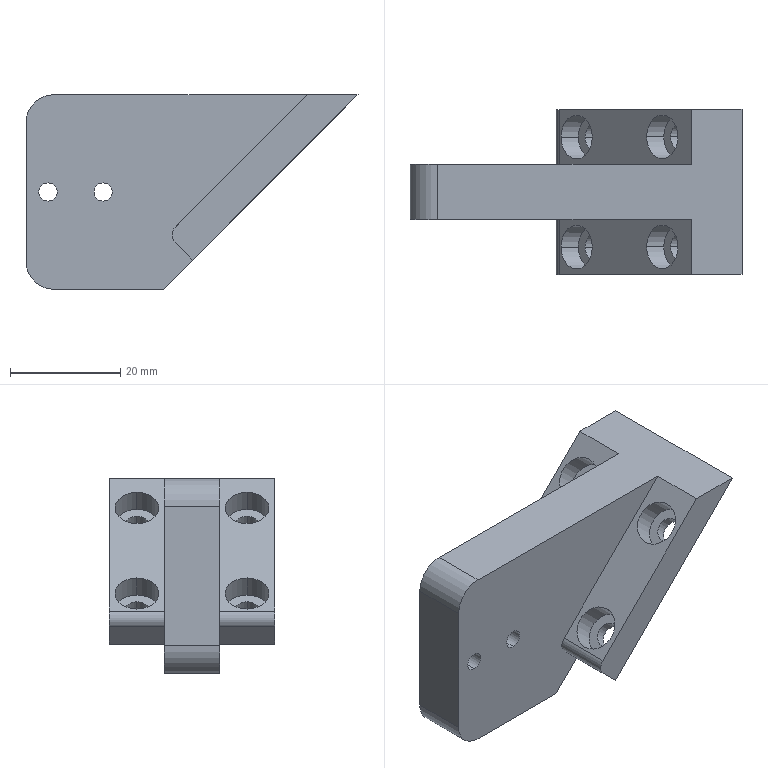Part | SolidWorks | features Fillet 2, HoleWzd 2, Extrusion 1, ICE 1, MirrorPattern 1 | 1 solid | 40 faces | box 60.355 x 30 x 35.355 mm | volume 18878 mm3 | cylinder 24 | plane 16 | commonest cylinder face diameters 4.5 x8 8 x8 3.3 x4 4 x2 10 x2
STEP:
#1=CARTESIAN_POINT('',(18.586,10.,-11.799));
#2=VERTEX_POINT('',#1);
#3=CARTESIAN_POINT('',(24.243,10.,-6.142));
#4=VERTEX_POINT('',#3);
#5=CARTESIAN_POINT('',(21.415,10.,-8.971));
#6=DIRECTION('',(-0.7071,0.,0.7071));
#7=DIRECTION('',(0.7071,0.,0.7071));
#8=AXIS2_PLACEMENT_3D('',#5,#6,#7);
#9=CIRCLE('',#8,4.);
#10=EDGE_CURVE('',#2,#4,#9,.T.);
#11=ORIENTED_EDGE('',*,*,#10,.F.);
#12=CARTESIAN_POINT('',(15.475,10.,-8.688));
#13=VERTEX_POINT('',#12);
#14=CARTESIAN_POINT('',(15.475,10.,-8.688));
#15=DIRECTION('',(-0.7071,0.,0.7071));
#16=VECTOR('',#15,1000.);
#17=LINE('',#14,#16);
#18=EDGE_CURVE('',#2,#13,#17,.T.);
#19=ORIENTED_EDGE('',*,*,#18,.T.);
#20=CARTESIAN_POINT('',(21.132,10.,-3.031));
#21=VERTEX_POINT('',#20);
#22=CARTESIAN_POINT('',(18.303,10.,-5.86));
#23=DIRECTION('',(-0.7071,0.,0.7071));
#24=DIRECTION('',(0.7071,0.,0.7071));
#25=AXIS2_PLACEMENT_3D('',#22,#23,#24);
#26=CIRCLE('',#25,4.);
#27=EDGE_CURVE('',#13,#21,#26,.T.);
#28=ORIENTED_EDGE('',*,*,#27,.T.);
#29=CARTESIAN_POINT('',(21.132,10.,-3.031));
#30=DIRECTION('',(-0.7071,0.,0.7071));
#31=VECTOR('',#30,1000.);
#32=LINE('',#29,#31);
#33=EDGE_CURVE('',#4,#21,#32,.T.);
#34=ORIENTED_EDGE('',*,*,#33,.F.);
#35=EDGE_LOOP('',(#11,#19,#28,#34));
#36=FACE_OUTER_BOUND('',#35,.T.);
#37=CARTESIAN_POINT('',(18.303,10.,-5.86));
#38=DIRECTION('',(-0.7071,0.,0.7071));
#39=DIRECTION('',(0.7071,0.,0.7071));
#40=AXIS2_PLACEMENT_3D('',#37,#38,#39);
#41=CYLINDRICAL_SURFACE('',#40,4.);
#42=ADVANCED_FACE('',(#36),#41,.F.);
#43=CARTESIAN_POINT('',(21.309,10.,-12.047));
#44=VERTEX_POINT('',#43);
#45=CARTESIAN_POINT('',(24.49,10.,-8.865));
#46=VERTEX_POINT('',#45);
#47=CARTESIAN_POINT('',(22.899,10.,-10.456));
#48=DIRECTION('',(-0.7071,0.,0.7071));
#49=DIRECTION('',(0.7071,0.,0.7071));
#50=AXIS2_PLACEMENT_3D('',#47,#48,#49);
#51=CIRCLE('',#50,2.25);
#52=EDGE_CURVE('',#44,#46,#51,.T.);
#53=ORIENTED_EDGE('',*,*,#52,.F.);
#54=CARTESIAN_POINT('',(19.824,10.,-10.562));
#55=VERTEX_POINT('',#54);
#56=CARTESIAN_POINT('',(16.712,10.,-7.451));
#57=DIRECTION('',(-0.7071,0.,0.7071));
#58=VECTOR('',#57,1000.);
#59=LINE('',#56,#58);
#60=EDGE_CURVE('',#44,#55,#59,.T.);
#61=ORIENTED_EDGE('',*,*,#60,.T.);
#62=CARTESIAN_POINT('',(23.006,10.,-7.38));
#63=VERTEX_POINT('',#62);
#64=CARTESIAN_POINT('',(21.415,10.,-8.971));
#65=DIRECTION('',(-0.7071,0.,0.7071));
#66=DIRECTION('',(0.7071,0.,0.7071));
#67=AXIS2_PLACEMENT_3D('',#64,#65,#66);
#68=CIRCLE('',#67,2.25);
#69=EDGE_CURVE('',#55,#63,#68,.T.);
#70=ORIENTED_EDGE('',*,*,#69,.T.);
#71=CARTESIAN_POINT('',(19.894,10.,-4.269));
#72=DIRECTION('',(-0.7071,0.,0.7071));
#73=VECTOR('',#72,1000.);
#74=LINE('',#71,#73);
#75=EDGE_CURVE('',#46,#63,#74,.T.);
#76=ORIENTED_EDGE('',*,*,#75,.F.);
#77=EDGE_LOOP('',(#53,#61,#70,#76));
#78=FACE_OUTER_BOUND('',#77,.T.);
#79=CARTESIAN_POINT('',(18.303,10.,-5.86));
#80=DIRECTION('',(-0.7071,0.,0.7071));
#81=DIRECTION('',(0.7071,0.,0.7071));
#82=AXIS2_PLACEMENT_3D('',#79,#80,#81);
#83=CYLINDRICAL_SURFACE('',#82,2.25);
#84=ADVANCED_FACE('',(#78),#83,.F.);
#85=CARTESIAN_POINT('',(34.142,10.,3.757));
#86=VERTEX_POINT('',#85);
#87=CARTESIAN_POINT('',(39.799,10.,9.414));
#88=VERTEX_POINT('',#87);
#89=CARTESIAN_POINT('',(36.971,10.,6.585));
#90=DIRECTION('',(-0.7071,0.,0.7071));
#91=DIRECTION('',(0.7071,0.,0.7071));
#92=AXIS2_PLACEMENT_3D('',#89,#90,#91);
#93=CIRCLE('',#92,4.);
#94=EDGE_CURVE('',#86,#88,#93,.T.);
#95=ORIENTED_EDGE('',*,*,#94,.F.);
#96=CARTESIAN_POINT('',(31.031,10.,6.868));
#97=VERTEX_POINT('',#96);
#98=CARTESIAN_POINT('',(31.031,10.,6.868));
#99=DIRECTION('',(-0.7071,0.,0.7071));
#100=VECTOR('',#99,1000.);
#101=LINE('',#98,#100);
#102=EDGE_CURVE('',#86,#97,#101,.T.);
#103=ORIENTED_EDGE('',*,*,#102,.T.);
#104=CARTESIAN_POINT('',(36.688,10.,12.525));
#105=VERTEX_POINT('',#104);
#106=CARTESIAN_POINT('',(33.86,10.,9.697));
#107=DIRECTION('',(-0.7071,0.,0.7071));
#108=DIRECTION('',(0.7071,0.,0.7071));
#109=AXIS2_PLACEMENT_3D('',#106,#107,#108);
#110=CIRCLE('',#109,4.);
#111=EDGE_CURVE('',#97,#105,#110,.T.);
#112=ORIENTED_EDGE('',*,*,#111,.T.);
#113=CARTESIAN_POINT('',(36.688,10.,12.525));
#114=DIRECTION('',(-0.7071,0.,0.7071));
#115=VECTOR('',#114,1000.);
#116=LINE('',#113,#115);
#117=EDGE_CURVE('',#88,#105,#116,.T.);
#118=ORIENTED_EDGE('',*,*,#117,.F.);
#119=EDGE_LOOP('',(#95,#103,#112,#118));
#120=FACE_OUTER_BOUND('',#119,.T.);
#121=CARTESIAN_POINT('',(33.86,10.,9.697));
#122=DIRECTION('',(-0.7071,0.,0.7071));
#123=DIRECTION('',(0.7071,0.,0.7071));
#124=AXIS2_PLACEMENT_3D('',#121,#122,#123);
#125=CYLINDRICAL_SURFACE('',#124,4.);
#126=ADVANCED_FACE('',(#120),#125,.F.);
#127=CARTESIAN_POINT('',(36.865,10.,3.51));
#128=VERTEX_POINT('',#127);
#129=CARTESIAN_POINT('',(40.047,10.,6.691));
#130=VERTEX_POINT('',#129);
#131=CARTESIAN_POINT('',(38.456,10.,5.101));
#132=DIRECTION('',(-0.7071,0.,0.7071));
#133=DIRECTION('',(0.7071,0.,0.7071));
#134=AXIS2_PLACEMENT_3D('',#131,#132,#133);
#135=CIRCLE('',#134,2.25);
#136=EDGE_CURVE('',#128,#130,#135,.T.);
#137=ORIENTED_EDGE('',*,*,#136,.F.);
#138=CARTESIAN_POINT('',(35.38,10.,4.994));
#139=VERTEX_POINT('',#138);
#140=CARTESIAN_POINT('',(32.269,10.,8.106));
#141=DIRECTION('',(-0.7071,0.,0.7071));
#142=VECTOR('',#141,1000.);
#143=LINE('',#140,#142);
#144=EDGE_CURVE('',#128,#139,#143,.T.);
#145=ORIENTED_EDGE('',*,*,#144,.T.);
#146=CARTESIAN_POINT('',(38.562,10.,8.176));
#147=VERTEX_POINT('',#146);
#148=CARTESIAN_POINT('',(36.971,10.,6.585));
#149=DIRECTION('',(-0.7071,0.,0.7071));
#150=DIRECTION('',(0.7071,0.,0.7071));
#151=AXIS2_PLACEMENT_3D('',#148,#149,#150);
#152=CIRCLE('',#151,2.25);
#153=EDGE_CURVE('',#139,#147,#152,.T.);
#154=ORIENTED_EDGE('',*,*,#153,.T.);
#155=CARTESIAN_POINT('',(35.451,10.,11.288));
#156=DIRECTION('',(-0.7071,0.,0.7071));
#157=VECTOR('',#156,1000.);
#158=LINE('',#155,#157);
#159=EDGE_CURVE('',#130,#147,#158,.T.);
#160=ORIENTED_EDGE('',*,*,#159,.F.);
#161=EDGE_LOOP('',(#137,#145,#154,#160));
#162=FACE_OUTER_BOUND('',#161,.T.);
#163=CARTESIAN_POINT('',(33.86,10.,9.697));
#164=DIRECTION('',(-0.7071,0.,0.7071));
#165=DIRECTION('',(0.7071,0.,0.7071));
#166=AXIS2_PLACEMENT_3D('',#163,#164,#165);
#167=CYLINDRICAL_SURFACE('',#166,2.25);
#168=ADVANCED_FACE('',(#162),#167,.F.);
#169=CARTESIAN_POINT('',(18.586,-10.,-11.799));
#170=VERTEX_POINT('',#169);
#171=CARTESIAN_POINT('',(24.243,-10.,-6.142));
#172=VERTEX_POINT('',#171);
#173=CARTESIAN_POINT('',(21.415,-10.,-8.971));
#174=DIRECTION('',(-0.7071,0.,0.7071));
#175=DIRECTION('',(0.7071,0.,0.7071));
#176=AXIS2_PLACEMENT_3D('',#173,#174,#175);
#177=CIRCLE('',#176,4.);
#178=EDGE_CURVE('',#170,#172,#177,.T.);
#179=ORIENTED_EDGE('',*,*,#178,.F.);
#180=CARTESIAN_POINT('',(15.475,-10.,-8.688));
#181=VERTEX_POINT('',#180);
#182=CARTESIAN_POINT('',(15.475,-10.,-8.688));
#183=DIRECTION('',(-0.7071,0.,0.7071));
#184=VECTOR('',#183,1000.);
#185=LINE('',#182,#184);
#186=EDGE_CURVE('',#170,#181,#185,.T.);
#187=ORIENTED_EDGE('',*,*,#186,.T.);
#188=CARTESIAN_POINT('',(21.132,-10.,-3.031));
#189=VERTEX_POINT('',#188);
#190=CARTESIAN_POINT('',(18.303,-10.,-5.86));
#191=DIRECTION('',(-0.7071,0.,0.7071));
#192=DIRECTION('',(0.7071,0.,0.7071));
#193=AXIS2_PLACEMENT_3D('',#190,#191,#192);
#194=CIRCLE('',#193,4.);
#195=EDGE_CURVE('',#181,#189,#194,.T.);
#196=ORIENTED_EDGE('',*,*,#195,.T.);
#197=CARTESIAN_POINT('',(21.132,-10.,-3.031));
#198=DIRECTION('',(-0.7071,0.,0.7071));
#199=VECTOR('',#198,1000.);
#200=LINE('',#197,#199);
#201=EDGE_CURVE('',#172,#189,#200,.T.);
#202=ORIENTED_EDGE('',*,*,#201,.F.);
#203=EDGE_LOOP('',(#179,#187,#196,#202));
#204=FACE_OUTER_BOUND('',#203,.T.);
#205=CARTESIAN_POINT('',(18.303,-10.,-5.86));
#206=DIRECTION('',(-0.7071,0.,0.7071));
#207=DIRECTION('',(0.7071,0.,0.7071));
#208=AXIS2_PLACEMENT_3D('',#205,#206,#207);
#209=CYLINDRICAL_SURFACE('',#208,4.);
#210=ADVANCED_FACE('',(#204),#209,.F.);
#211=CARTESIAN_POINT('',(21.309,-10.,-12.047));
#212=VERTEX_POINT('',#211);
#213=CARTESIAN_POINT('',(24.49,-10.,-8.865));
#214=VERTEX_POINT('',#213);
#215=CARTESIAN_POINT('',(22.899,-10.,-10.456));
#216=DIRECTION('',(-0.7071,0.,0.7071));
#217=DIRECTION('',(0.7071,0.,0.7071));
#218=AXIS2_PLACEMENT_3D('',#215,#216,#217);
#219=CIRCLE('',#218,2.25);
#220=EDGE_CURVE('',#212,#214,#219,.T.);
#221=ORIENTED_EDGE('',*,*,#220,.F.);
#222=CARTESIAN_POINT('',(19.824,-10.,-10.562));
#223=VERTEX_POINT('',#222);
#224=CARTESIAN_POINT('',(16.712,-10.,-7.451));
#225=DIRECTION('',(-0.7071,0.,0.7071));
#226=VECTOR('',#225,1000.);
#227=LINE('',#224,#226);
#228=EDGE_CURVE('',#212,#223,#227,.T.);
#229=ORIENTED_EDGE('',*,*,#228,.T.);
#230=CARTESIAN_POINT('',(23.006,-10.,-7.38));
#231=VERTEX_POINT('',#230);
#232=CARTESIAN_POINT('',(21.415,-10.,-8.971));
#233=DIRECTION('',(-0.7071,0.,0.7071));
#234=DIRECTION('',(0.7071,0.,0.7071));
#235=AXIS2_PLACEMENT_3D('',#232,#233,#234);
#236=CIRCLE('',#235,2.25);
#237=EDGE_CURVE('',#223,#231,#236,.T.);
#238=ORIENTED_EDGE('',*,*,#237,.T.);
#239=CARTESIAN_POINT('',(19.894,-10.,-4.269));
#240=DIRECTION('',(-0.7071,0.,0.7071));
#241=VECTOR('',#240,1000.);
#242=LINE('',#239,#241);
#243=EDGE_CURVE('',#214,#231,#242,.T.);
#244=ORIENTED_EDGE('',*,*,#243,.F.);
#245=EDGE_LOOP('',(#221,#229,#238,#244));
#246=FACE_OUTER_BOUND('',#245,.T.);
#247=CARTESIAN_POINT('',(18.303,-10.,-5.86));
#248=DIRECTION('',(-0.7071,0.,0.7071));
#249=DIRECTION('',(0.7071,0.,0.7071));
#250=AXIS2_PLACEMENT_3D('',#247,#248,#249);
#251=CYLINDRICAL_SURFACE('',#250,2.25);
#252=ADVANCED_FACE('',(#246),#251,.F.);
#253=CARTESIAN_POINT('',(34.142,-10.,3.757));
#254=VERTEX_POINT('',#253);
#255=CARTESIAN_POINT('',(39.799,-10.,9.414));
#256=VERTEX_POINT('',#255);
#257=CARTESIAN_POINT('',(36.971,-10.,6.585));
#258=DIRECTION('',(-0.7071,0.,0.7071));
#259=DIRECTION('',(0.7071,0.,0.7071));
#260=AXIS2_PLACEMENT_3D('',#257,#258,#259);
#261=CIRCLE('',#260,4.);
#262=EDGE_CURVE('',#254,#256,#261,.T.);
#263=ORIENTED_EDGE('',*,*,#262,.F.);
#264=CARTESIAN_POINT('',(31.031,-10.,6.868));
#265=VERTEX_POINT('',#264);
#266=CARTESIAN_POINT('',(31.031,-10.,6.868));
#267=DIRECTION('',(-0.7071,0.,0.7071));
#268=VECTOR('',#267,1000.);
#269=LINE('',#266,#268);
#270=EDGE_CURVE('',#254,#265,#269,.T.);
#271=ORIENTED_EDGE('',*,*,#270,.T.);
#272=CARTESIAN_POINT('',(36.688,-10.,12.525));
#273=VERTEX_POINT('',#272);
#274=CARTESIAN_POINT('',(33.86,-10.,9.697));
#275=DIRECTION('',(-0.7071,0.,0.7071));
#276=DIRECTION('',(0.7071,0.,0.7071));
#277=AXIS2_PLACEMENT_3D('',#274,#275,#276);
#278=CIRCLE('',#277,4.);
#279=EDGE_CURVE('',#265,#273,#278,.T.);
#280=ORIENTED_EDGE('',*,*,#279,.T.);
#281=CARTESIAN_POINT('',(36.688,-10.,12.525));
#282=DIRECTION('',(-0.7071,0.,0.7071));
#283=VECTOR('',#282,1000.);
#284=LINE('',#281,#283);
#285=EDGE_CURVE('',#256,#273,#284,.T.);
#286=ORIENTED_EDGE('',*,*,#285,.F.);
#287=EDGE_LOOP('',(#263,#271,#280,#286));
#288=FACE_OUTER_BOUND('',#287,.T.);
#289=CARTESIAN_POINT('',(33.86,-10.,9.697));
#290=DIRECTION('',(-0.7071,0.,0.7071));
#291=DIRECTION('',(0.7071,0.,0.7071));
#292=AXIS2_PLACEMENT_3D('',#289,#290,#291);
#293=CYLINDRICAL_SURFACE('',#292,4.);
#294=ADVANCED_FACE('',(#288),#293,.F.);
#295=CARTESIAN_POINT('',(36.865,-10.,3.51));
#296=VERTEX_POINT('',#295);
#297=CARTESIAN_POINT('',(40.047,-10.,6.691));
#298=VERTEX_POINT('',#297);
#299=CARTESIAN_POINT('',(38.456,-10.,5.101));
#300=DIRECTION('',(-0.7071,0.,0.7071));
#301=DIRECTION('',(0.7071,0.,0.7071));
#302=AXIS2_PLACEMENT_3D('',#299,#300,#301);
#303=CIRCLE('',#302,2.25);
#304=EDGE_CURVE('',#296,#298,#303,.T.);
#305=ORIENTED_EDGE('',*,*,#304,.F.);
#306=CARTESIAN_POINT('',(35.38,-10.,4.994));
#307=VERTEX_POINT('',#306);
#308=CARTESIAN_POINT('',(32.269,-10.,8.106));
#309=DIRECTION('',(-0.7071,0.,0.7071));
#310=VECTOR('',#309,1000.);
#311=LINE('',#308,#310);
#312=EDGE_CURVE('',#296,#307,#311,.T.);
#313=ORIENTED_EDGE('',*,*,#312,.T.);
#314=CARTESIAN_POINT('',(38.562,-10.,8.176));
#315=VERTEX_POINT('',#314);
#316=CARTESIAN_POINT('',(36.971,-10.,6.585));
#317=DIRECTION('',(-0.7071,0.,0.7071));
#318=DIRECTION('',(0.7071,0.,0.7071));
#319=AXIS2_PLACEMENT_3D('',#316,#317,#318);
#320=CIRCLE('',#319,2.25);
#321=EDGE_CURVE('',#307,#315,#320,.T.);
#322=ORIENTED_EDGE('',*,*,#321,.T.);
#323=CARTESIAN_POINT('',(35.451,-10.,11.288));
#324=DIRECTION('',(-0.7071,0.,0.7071));
#325=VECTOR('',#324,1000.);
#326=LINE('',#323,#325);
#327=EDGE_CURVE('',#298,#315,#326,.T.);
#328=ORIENTED_EDGE('',*,*,#327,.F.);
#329=EDGE_LOOP('',(#305,#313,#322,#328));
#330=FACE_OUTER_BOUND('',#329,.T.);
#331=CARTESIAN_POINT('',(33.86,-10.,9.697));
#332=DIRECTION('',(-0.7071,0.,0.7071));
#333=DIRECTION('',(0.7071,0.,0.7071));
#334=AXIS2_PLACEMENT_3D('',#331,#332,#333);
#335=CYLINDRICAL_SURFACE('',#334,2.25);
#336=ADVANCED_FACE('',(#330),#335,.F.);
#337=CARTESIAN_POINT('',(-8.,5.,-1.028));
#338=VERTEX_POINT('',#337);
#339=CARTESIAN_POINT('',(-8.,5.,-4.328));
#340=VERTEX_POINT('',#339);
#341=CARTESIAN_POINT('',(-8.,5.,-2.678));
#342=DIRECTION('',(0.,-1.,0.));
#343=DIRECTION('',(0.,0.,-1.));
#344=AXIS2_PLACEMENT_3D('',#341,#342,#343);
#345=CIRCLE('',#344,1.65);
#346=EDGE_CURVE('',#338,#340,#345,.T.);
#347=ORIENTED_EDGE('',*,*,#346,.F.);
#348=CARTESIAN_POINT('',(-8.,-5.,-1.028));
#349=VERTEX_POINT('',#348);
#350=CARTESIAN_POINT('',(-8.,-5.,-1.028));
#351=DIRECTION('',(0.,-1.,0.));
#352=VECTOR('',#351,1000.);
#353=LINE('',#350,#352);
#354=EDGE_CURVE('',#338,#349,#353,.T.);
#355=ORIENTED_EDGE('',*,*,#354,.T.);
#356=CARTESIAN_POINT('',(-8.,-5.,-4.328));
#357=VERTEX_POINT('',#356);
#358=CARTESIAN_POINT('',(-8.,-5.,-2.678));
#359=DIRECTION('',(0.,-1.,0.));
#360=DIRECTION('',(0.,0.,-1.));
#361=AXIS2_PLACEMENT_3D('',#358,#359,#360);
#362=CIRCLE('',#361,1.65);
#363=EDGE_CURVE('',#349,#357,#362,.T.);
#364=ORIENTED_EDGE('',*,*,#363,.T.);
#365=CARTESIAN_POINT('',(-8.,-5.,-4.328));
#366=DIRECTION('',(0.,-1.,0.));
#367=VECTOR('',#366,1000.);
#368=LINE('',#365,#367);
#369=EDGE_CURVE('',#340,#357,#368,.T.);
#370=ORIENTED_EDGE('',*,*,#369,.F.);
#371=EDGE_LOOP('',(#347,#355,#364,#370));
#372=FACE_OUTER_BOUND('',#371,.T.);
#373=CARTESIAN_POINT('',(-8.,-5.,-2.678));
#374=DIRECTION('',(0.,-1.,0.));
#375=DIRECTION('',(0.,0.,-1.));
#376=AXIS2_PLACEMENT_3D('',#373,#374,#375);
#377=CYLINDRICAL_SURFACE('',#376,1.65);
#378=ADVANCED_FACE('',(#372),#377,.F.);
#379=CARTESIAN_POINT('',(2.,5.,-1.028));
#380=VERTEX_POINT('',#379);
#381=CARTESIAN_POINT('',(2.,5.,-4.328));
#382=VERTEX_POINT('',#381);
#383=CARTESIAN_POINT('',(2.,5.,-2.678));
#384=DIRECTION('',(0.,-1.,0.));
#385=DIRECTION('',(0.,0.,-1.));
#386=AXIS2_PLACEMENT_3D('',#383,#384,#385);
#387=CIRCLE('',#386,1.65);
#388=EDGE_CURVE('',#380,#382,#387,.T.);
#389=ORIENTED_EDGE('',*,*,#388,.F.);
#390=CARTESIAN_POINT('',(2.,-5.,-1.028));
#391=VERTEX_POINT('',#390);
#392=CARTESIAN_POINT('',(2.,-5.,-1.028));
#393=DIRECTION('',(0.,-1.,0.));
#394=VECTOR('',#393,1000.);
#395=LINE('',#392,#394);
#396=EDGE_CURVE('',#380,#391,#395,.T.);
#397=ORIENTED_EDGE('',*,*,#396,.T.);
#398=CARTESIAN_POINT('',(2.,-5.,-4.328));
#399=VERTEX_POINT('',#398);
#400=CARTESIAN_POINT('',(2.,-5.,-2.678));
#401=DIRECTION('',(0.,-1.,0.));
#402=DIRECTION('',(0.,0.,-1.));
#403=AXIS2_PLACEMENT_3D('',#400,#401,#402);
#404=CIRCLE('',#403,1.65);
#405=EDGE_CURVE('',#391,#399,#404,.T.);
#406=ORIENTED_EDGE('',*,*,#405,.T.);
#407=CARTESIAN_POINT('',(2.,-5.,-4.328));
#408=DIRECTION('',(0.,-1.,0.));
#409=VECTOR('',#408,1000.);
#410=LINE('',#407,#409);
#411=EDGE_CURVE('',#382,#399,#410,.T.);
#412=ORIENTED_EDGE('',*,*,#411,.F.);
#413=EDGE_LOOP('',(#389,#397,#406,#412));
#414=FACE_OUTER_BOUND('',#413,.T.);
#415=CARTESIAN_POINT('',(2.,-5.,-2.678));
#416=DIRECTION('',(0.,-1.,0.));
#417=DIRECTION('',(0.,0.,-1.));
#418=AXIS2_PLACEMENT_3D('',#415,#416,#417);
#419=CYLINDRICAL_SURFACE('',#418,1.65);
#420=ADVANCED_FACE('',(#414),#419,.F.);
#421=CARTESIAN_POINT('',(-8.,5.,-2.678));
#422=DIRECTION('',(0.,-1.,0.));
#423=DIRECTION('',(0.,0.,-1.));
#424=AXIS2_PLACEMENT_3D('',#421,#422,#423);
#425=CIRCLE('',#424,1.65);
#426=EDGE_CURVE('',#340,#338,#425,.T.);
#427=ORIENTED_EDGE('',*,*,#426,.T.);
#428=ORIENTED_EDGE('',*,*,#346,.T.);
#429=EDGE_LOOP('',(#427,#428));
#430=FACE_BOUND('',#429,.T.);
#431=CARTESIAN_POINT('',(2.,5.,-2.678));
#432=DIRECTION('',(0.,-1.,0.));
#433=DIRECTION('',(0.,0.,-1.));
#434=AXIS2_PLACEMENT_3D('',#431,#432,#433);
#435=CIRCLE('',#434,1.65);
#436=EDGE_CURVE('',#382,#380,#435,.T.);
#437=ORIENTED_EDGE('',*,*,#436,.T.);
#438=ORIENTED_EDGE('',*,*,#388,.T.);
#439=EDGE_LOOP('',(#437,#438));
#440=FACE_BOUND('',#439,.T.);
#441=CARTESIAN_POINT('',(-12.,5.,-15.355));
#442=VERTEX_POINT('',#441);
#443=CARTESIAN_POINT('',(-12.,5.,10.));
#444=VERTEX_POINT('',#443);
#445=CARTESIAN_POINT('',(-12.,5.,-20.355));
#446=DIRECTION('',(0.,0.,1.));
#447=VECTOR('',#446,1000.);
#448=LINE('',#445,#447);
#449=EDGE_CURVE('',#442,#444,#448,.T.);
#450=ORIENTED_EDGE('',*,*,#449,.T.);
#451=CARTESIAN_POINT('',(-7.,5.,15.));
#452=VERTEX_POINT('',#451);
#453=CARTESIAN_POINT('',(-7.,5.,10.));
#454=DIRECTION('',(0.,1.,0.));
#455=DIRECTION('',(0.,0.,1.));
#456=AXIS2_PLACEMENT_3D('',#453,#454,#455);
#457=CIRCLE('',#456,5.);
#458=EDGE_CURVE('',#444,#452,#457,.T.);
#459=ORIENTED_EDGE('',*,*,#458,.T.);
#460=CARTESIAN_POINT('',(39.163,5.,15.));
#461=VERTEX_POINT('',#460);
#462=CARTESIAN_POINT('',(-12.,5.,15.));
#463=DIRECTION('',(1.,0.,0.));
#464=VECTOR('',#463,1000.);
#465=LINE('',#462,#464);
#466=EDGE_CURVE('',#452,#461,#465,.T.);
#467=ORIENTED_EDGE('',*,*,#466,.T.);
#468=CARTESIAN_POINT('',(15.121,5.,-9.042));
#469=VERTEX_POINT('',#468);
#470=CARTESIAN_POINT('',(13.707,5.,-10.456));
#471=DIRECTION('',(-0.7071,0.,-0.7071));
#472=VECTOR('',#471,1000.);
#473=LINE('',#470,#472);
#474=EDGE_CURVE('',#461,#469,#473,.T.);
#475=ORIENTED_EDGE('',*,*,#474,.T.);
#476=CARTESIAN_POINT('',(15.121,5.,-11.87));
#477=VERTEX_POINT('',#476);
#478=CARTESIAN_POINT('',(16.536,5.,-10.456));
#479=DIRECTION('',(0.,-1.,0.));
#480=DIRECTION('',(0.,0.,1.));
#481=AXIS2_PLACEMENT_3D('',#478,#479,#480);
#482=CIRCLE('',#481,2.);
#483=EDGE_CURVE('',#469,#477,#482,.T.);
#484=ORIENTED_EDGE('',*,*,#483,.T.);
#485=CARTESIAN_POINT('',(18.303,5.,-15.052));
#486=VERTEX_POINT('',#485);
#487=CARTESIAN_POINT('',(18.303,5.,-15.052));
#488=DIRECTION('',(0.7071,0.,-0.7071));
#489=VECTOR('',#488,1000.);
#490=LINE('',#487,#489);
#491=EDGE_CURVE('',#477,#486,#490,.T.);
#492=ORIENTED_EDGE('',*,*,#491,.T.);
#493=CARTESIAN_POINT('',(13.,5.,-20.355));
#494=VERTEX_POINT('',#493);
#495=CARTESIAN_POINT('',(48.355,5.,15.));
#496=DIRECTION('',(-0.7071,0.,-0.7071));
#497=VECTOR('',#496,1000.);
#498=LINE('',#495,#497);
#499=EDGE_CURVE('',#486,#494,#498,.T.);
#500=ORIENTED_EDGE('',*,*,#499,.T.);
#501=CARTESIAN_POINT('',(-7.,5.,-20.355));
#502=VERTEX_POINT('',#501);
#503=CARTESIAN_POINT('',(13.,5.,-20.355));
#504=DIRECTION('',(-1.,0.,0.));
#505=VECTOR('',#504,1000.);
#506=LINE('',#503,#505);
#507=EDGE_CURVE('',#494,#502,#506,.T.);
#508=ORIENTED_EDGE('',*,*,#507,.T.);
#509=CARTESIAN_POINT('',(-7.,5.,-15.355));
#510=DIRECTION('',(0.,1.,0.));
#511=DIRECTION('',(0.,0.,1.));
#512=AXIS2_PLACEMENT_3D('',#509,#510,#511);
#513=CIRCLE('',#512,5.);
#514=EDGE_CURVE('',#502,#442,#513,.T.);
#515=ORIENTED_EDGE('',*,*,#514,.T.);
#516=EDGE_LOOP('',(#450,#459,#467,#475,#484,#492,#500,#508,#515));
#517=FACE_OUTER_BOUND('',#516,.T.);
#518=CARTESIAN_POINT('',(0.,5.,0.));
#519=DIRECTION('',(0.,1.,0.));
#520=DIRECTION('',(0.,0.,1.));
#521=AXIS2_PLACEMENT_3D('',#518,#519,#520);
#522=PLANE('',#521);
#523=ADVANCED_FACE('',(#430,#440,#517),#522,.T.);
#524=CARTESIAN_POINT('',(2.,-5.,-2.678));
#525=DIRECTION('',(0.,-1.,0.));
#526=DIRECTION('',(0.,0.,-1.));
#527=AXIS2_PLACEMENT_3D('',#524,#525,#526);
#528=CIRCLE('',#527,1.65);
#529=EDGE_CURVE('',#399,#391,#528,.T.);
#530=ORIENTED_EDGE('',*,*,#529,.F.);
#531=ORIENTED_EDGE('',*,*,#405,.F.);
#532=EDGE_LOOP('',(#530,#531));
#533=FACE_BOUND('',#532,.T.);
#534=CARTESIAN_POINT('',(-8.,-5.,-2.678));
#535=DIRECTION('',(0.,-1.,0.));
#536=DIRECTION('',(0.,0.,-1.));
#537=AXIS2_PLACEMENT_3D('',#534,#535,#536);
#538=CIRCLE('',#537,1.65);
#539=EDGE_CURVE('',#357,#349,#538,.T.);
#540=ORIENTED_EDGE('',*,*,#539,.F.);
#541=ORIENTED_EDGE('',*,*,#363,.F.);
#542=EDGE_LOOP('',(#540,#541));
#543=FACE_BOUND('',#542,.T.);
#544=CARTESIAN_POINT('',(-7.,-5.,15.));
#545=VERTEX_POINT('',#544);
#546=CARTESIAN_POINT('',(39.163,-5.,15.));
#547=VERTEX_POINT('',#546);
#548=CARTESIAN_POINT('',(-12.,-5.,15.));
#549=DIRECTION('',(1.,0.,0.));
#550=VECTOR('',#549,1000.);
#551=LINE('',#548,#550);
#552=EDGE_CURVE('',#545,#547,#551,.T.);
#553=ORIENTED_EDGE('',*,*,#552,.F.);
#554=CARTESIAN_POINT('',(-12.,-5.,10.));
#555=VERTEX_POINT('',#554);
#556=CARTESIAN_POINT('',(-7.,-5.,10.));
#557=DIRECTION('',(0.,-1.,0.));
#558=DIRECTION('',(0.,0.,1.));
#559=AXIS2_PLACEMENT_3D('',#556,#557,#558);
#560=CIRCLE('',#559,5.);
#561=EDGE_CURVE('',#545,#555,#560,.T.);
#562=ORIENTED_EDGE('',*,*,#561,.T.);
#563=CARTESIAN_POINT('',(-12.,-5.,-15.355));
#564=VERTEX_POINT('',#563);
#565=CARTESIAN_POINT('',(-12.,-5.,-20.355));
#566=DIRECTION('',(0.,0.,1.));
#567=VECTOR('',#566,1000.);
#568=LINE('',#565,#567);
#569=EDGE_CURVE('',#564,#555,#568,.T.);
#570=ORIENTED_EDGE('',*,*,#569,.F.);
#571=CARTESIAN_POINT('',(-7.,-5.,-20.355));
#572=VERTEX_POINT('',#571);
#573=CARTESIAN_POINT('',(-7.,-5.,-15.355));
#574=DIRECTION('',(0.,-1.,0.));
#575=DIRECTION('',(0.,0.,1.));
#576=AXIS2_PLACEMENT_3D('',#573,#574,#575);
#577=CIRCLE('',#576,5.);
#578=EDGE_CURVE('',#564,#572,#577,.T.);
#579=ORIENTED_EDGE('',*,*,#578,.T.);
#580=CARTESIAN_POINT('',(13.,-5.,-20.355));
#581=VERTEX_POINT('',#580);
#582=CARTESIAN_POINT('',(13.,-5.,-20.355));
#583=DIRECTION('',(-1.,0.,0.));
#584=VECTOR('',#583,1000.);
#585=LINE('',#582,#584);
#586=EDGE_CURVE('',#581,#572,#585,.T.);
#587=ORIENTED_EDGE('',*,*,#586,.F.);
#588=CARTESIAN_POINT('',(18.303,-5.,-15.052));
#589=VERTEX_POINT('',#588);
#590=CARTESIAN_POINT('',(48.355,-5.,15.));
#591=DIRECTION('',(-0.7071,0.,-0.7071));
#592=VECTOR('',#591,1000.);
#593=LINE('',#590,#592);
#594=EDGE_CURVE('',#589,#581,#593,.T.);
#595=ORIENTED_EDGE('',*,*,#594,.F.);
#596=CARTESIAN_POINT('',(15.121,-5.,-11.87));
#597=VERTEX_POINT('',#596);
#598=CARTESIAN_POINT('',(18.303,-5.,-15.052));
#599=DIRECTION('',(0.7071,0.,-0.7071));
#600=VECTOR('',#599,1000.);
#601=LINE('',#598,#600);
#602=EDGE_CURVE('',#597,#589,#601,.T.);
#603=ORIENTED_EDGE('',*,*,#602,.F.);
#604=CARTESIAN_POINT('',(15.121,-5.,-9.042));
#605=VERTEX_POINT('',#604);
#606=CARTESIAN_POINT('',(16.536,-5.,-10.456));
#607=DIRECTION('',(0.,1.,0.));
#608=DIRECTION('',(0.,0.,1.));
#609=AXIS2_PLACEMENT_3D('',#606,#607,#608);
#610=CIRCLE('',#609,2.);
#611=EDGE_CURVE('',#597,#605,#610,.T.);
#612=ORIENTED_EDGE('',*,*,#611,.T.);
#613=CARTESIAN_POINT('',(13.707,-5.,-10.456));
#614=DIRECTION('',(-0.7071,0.,-0.7071));
#615=VECTOR('',#614,1000.);
#616=LINE('',#613,#615);
#617=EDGE_CURVE('',#547,#605,#616,.T.);
#618=ORIENTED_EDGE('',*,*,#617,.F.);
#619=EDGE_LOOP('',(#553,#562,#570,#579,#587,#595,#603,#612,#618));
#620=FACE_OUTER_BOUND('',#619,.T.);
#621=CARTESIAN_POINT('',(0.,-5.,0.));
#622=DIRECTION('',(0.,1.,0.));
#623=DIRECTION('',(0.,0.,1.));
#624=AXIS2_PLACEMENT_3D('',#621,#622,#623);
#625=PLANE('',#624);
#626=ADVANCED_FACE('',(#533,#543,#620),#625,.F.);
#627=ORIENTED_EDGE('',*,*,#586,.T.);
#628=CARTESIAN_POINT('',(-7.,5.,-20.355));
#629=DIRECTION('',(0.,1.,0.));
#630=VECTOR('',#629,1000.);
#631=LINE('',#628,#630);
#632=EDGE_CURVE('',#572,#502,#631,.T.);
#633=ORIENTED_EDGE('',*,*,#632,.T.);
#634=ORIENTED_EDGE('',*,*,#507,.F.);
#635=CARTESIAN_POINT('',(13.,5.,-20.355));
#636=DIRECTION('',(0.,-1.,0.));
#637=VECTOR('',#636,1000.);
#638=LINE('',#635,#637);
#639=EDGE_CURVE('',#494,#581,#638,.T.);
#640=ORIENTED_EDGE('',*,*,#639,.T.);
#641=EDGE_LOOP('',(#627,#633,#634,#640));
#642=FACE_OUTER_BOUND('',#641,.T.);
#643=CARTESIAN_POINT('',(13.,5.,-20.355));
#644=DIRECTION('',(0.,0.,1.));
#645=DIRECTION('',(1.,0.,0.));
#646=AXIS2_PLACEMENT_3D('',#643,#644,#645);
#647=PLANE('',#646);
#648=ADVANCED_FACE('',(#642),#647,.F.);
#649=ORIENTED_EDGE('',*,*,#569,.T.);
#650=CARTESIAN_POINT('',(-12.,5.,10.));
#651=DIRECTION('',(0.,1.,0.));
#652=VECTOR('',#651,1000.);
#653=LINE('',#650,#652);
#654=EDGE_CURVE('',#555,#444,#653,.T.);
#655=ORIENTED_EDGE('',*,*,#654,.T.);
#656=ORIENTED_EDGE('',*,*,#449,.F.);
#657=CARTESIAN_POINT('',(-12.,5.,-15.355));
#658=DIRECTION('',(0.,-1.,0.));
#659=VECTOR('',#658,1000.);
#660=LINE('',#657,#659);
#661=EDGE_CURVE('',#442,#564,#660,.T.);
#662=ORIENTED_EDGE('',*,*,#661,.T.);
#663=EDGE_LOOP('',(#649,#655,#656,#662));
#664=FACE_OUTER_BOUND('',#663,.T.);
#665=CARTESIAN_POINT('',(-12.,5.,-20.355));
#666=DIRECTION('',(1.,0.,0.));
#667=DIRECTION('',(0.,0.,-1.));
#668=AXIS2_PLACEMENT_3D('',#665,#666,#667);
#669=PLANE('',#668);
#670=ADVANCED_FACE('',(#664),#669,.F.);
#671=ORIENTED_EDGE('',*,*,#466,.F.);
#672=CARTESIAN_POINT('',(-7.,5.,15.));
#673=DIRECTION('',(0.,-1.,0.));
#674=VECTOR('',#673,1000.);
#675=LINE('',#672,#674);
#676=EDGE_CURVE('',#452,#545,#675,.T.);
#677=ORIENTED_EDGE('',*,*,#676,.T.);
#678=ORIENTED_EDGE('',*,*,#552,.T.);
#679=CARTESIAN_POINT('',(39.163,-15.,15.));
#680=VERTEX_POINT('',#679);
#681=CARTESIAN_POINT('',(39.163,-15.,15.));
#682=DIRECTION('',(0.,1.,0.));
#683=VECTOR('',#682,1000.);
#684=LINE('',#681,#683);
#685=EDGE_CURVE('',#680,#547,#684,.T.);
#686=ORIENTED_EDGE('',*,*,#685,.F.);
#687=CARTESIAN_POINT('',(48.355,-15.,15.));
#688=VERTEX_POINT('',#687);
#689=CARTESIAN_POINT('',(39.163,-15.,15.));
#690=DIRECTION('',(-1.,0.,0.));
#691=VECTOR('',#690,1000.);
#692=LINE('',#689,#691);
#693=EDGE_CURVE('',#688,#680,#692,.T.);
#694=ORIENTED_EDGE('',*,*,#693,.F.);
#695=CARTESIAN_POINT('',(48.355,15.,15.));
#696=VERTEX_POINT('',#695);
#697=CARTESIAN_POINT('',(48.355,5.,15.));
#698=DIRECTION('',(0.,-1.,0.));
#699=VECTOR('',#698,1000.);
#700=LINE('',#697,#699);
#701=EDGE_CURVE('',#696,#688,#700,.T.);
#702=ORIENTED_EDGE('',*,*,#701,.F.);
#703=CARTESIAN_POINT('',(39.163,15.,15.));
#704=VERTEX_POINT('',#703);
#705=CARTESIAN_POINT('',(39.163,15.,15.));
#706=DIRECTION('',(-1.,0.,0.));
#707=VECTOR('',#706,1000.);
#708=LINE('',#705,#707);
#709=EDGE_CURVE('',#696,#704,#708,.T.);
#710=ORIENTED_EDGE('',*,*,#709,.T.);
#711=CARTESIAN_POINT('',(39.163,15.,15.));
#712=DIRECTION('',(0.,-1.,0.));
#713=VECTOR('',#712,1000.);
#714=LINE('',#711,#713);
#715=EDGE_CURVE('',#704,#461,#714,.T.);
#716=ORIENTED_EDGE('',*,*,#715,.T.);
#717=EDGE_LOOP('',(#671,#677,#678,#686,#694,#702,#710,#716));
#718=FACE_OUTER_BOUND('',#717,.T.);
#719=CARTESIAN_POINT('',(-12.,5.,15.));
#720=DIRECTION('',(0.,0.,-1.));
#721=DIRECTION('',(-1.,0.,0.));
#722=AXIS2_PLACEMENT_3D('',#719,#720,#721);
#723=PLANE('',#722);
#724=ADVANCED_FACE('',(#718),#723,.F.);
#725=CARTESIAN_POINT('',(22.899,10.,-10.456));
#726=DIRECTION('',(-0.7071,0.,0.7071));
#727=DIRECTION('',(0.7071,0.,0.7071));
#728=AXIS2_PLACEMENT_3D('',#725,#726,#727);
#729=CIRCLE('',#728,2.25);
#730=EDGE_CURVE('',#46,#44,#729,.T.);
#731=ORIENTED_EDGE('',*,*,#730,.T.);
#732=ORIENTED_EDGE('',*,*,#52,.T.);
#733=EDGE_LOOP('',(#731,#732));
#734=FACE_BOUND('',#733,.T.);
#735=CARTESIAN_POINT('',(38.456,10.,5.101));
#736=DIRECTION('',(-0.7071,0.,0.7071));
#737=DIRECTION('',(0.7071,0.,0.7071));
#738=AXIS2_PLACEMENT_3D('',#735,#736,#737);
#739=CIRCLE('',#738,2.25);
#740=EDGE_CURVE('',#130,#128,#739,.T.);
#741=ORIENTED_EDGE('',*,*,#740,.T.);
#742=ORIENTED_EDGE('',*,*,#136,.T.);
#743=EDGE_LOOP('',(#741,#742));
#744=FACE_BOUND('',#743,.T.);
#745=CARTESIAN_POINT('',(22.899,-10.,-10.456));
#746=DIRECTION('',(-0.7071,0.,0.7071));
#747=DIRECTION('',(0.7071,0.,0.7071));
#748=AXIS2_PLACEMENT_3D('',#745,#746,#747);
#749=CIRCLE('',#748,2.25);
#750=EDGE_CURVE('',#214,#212,#749,.T.);
#751=ORIENTED_EDGE('',*,*,#750,.T.);
#752=ORIENTED_EDGE('',*,*,#220,.T.);
#753=EDGE_LOOP('',(#751,#752));
#754=FACE_BOUND('',#753,.T.);
#755=CARTESIAN_POINT('',(38.456,-10.,5.101));
#756=DIRECTION('',(-0.7071,0.,0.7071));
#757=DIRECTION('',(0.7071,0.,0.7071));
#758=AXIS2_PLACEMENT_3D('',#755,#756,#757);
#759=CIRCLE('',#758,2.25);
#760=EDGE_CURVE('',#298,#296,#759,.T.);
#761=ORIENTED_EDGE('',*,*,#760,.T.);
#762=ORIENTED_EDGE('',*,*,#304,.T.);
#763=EDGE_LOOP('',(#761,#762));
#764=FACE_BOUND('',#763,.T.);
#765=ORIENTED_EDGE('',*,*,#701,.T.);
#766=CARTESIAN_POINT('',(18.303,-15.,-15.052));
#767=VERTEX_POINT('',#766);
#768=CARTESIAN_POINT('',(48.355,-15.,15.));
#769=DIRECTION('',(0.7071,0.,0.7071));
#770=VECTOR('',#769,1000.);
#771=LINE('',#768,#770);
#772=EDGE_CURVE('',#767,#688,#771,.T.);
#773=ORIENTED_EDGE('',*,*,#772,.F.);
#774=CARTESIAN_POINT('',(18.303,-15.,-15.052));
#775=DIRECTION('',(0.,1.,0.));
#776=VECTOR('',#775,1000.);
#777=LINE('',#774,#776);
#778=EDGE_CURVE('',#767,#589,#777,.T.);
#779=ORIENTED_EDGE('',*,*,#778,.T.);
#780=ORIENTED_EDGE('',*,*,#594,.T.);
#781=ORIENTED_EDGE('',*,*,#639,.F.);
#782=ORIENTED_EDGE('',*,*,#499,.F.);
#783=CARTESIAN_POINT('',(18.303,15.,-15.052));
#784=VERTEX_POINT('',#783);
#785=CARTESIAN_POINT('',(18.303,15.,-15.052));
#786=DIRECTION('',(0.,-1.,0.));
#787=VECTOR('',#786,1000.);
#788=LINE('',#785,#787);
#789=EDGE_CURVE('',#784,#486,#788,.T.);
#790=ORIENTED_EDGE('',*,*,#789,.F.);
#791=CARTESIAN_POINT('',(48.355,15.,15.));
#792=DIRECTION('',(0.7071,0.,0.7071));
#793=VECTOR('',#792,1000.);
#794=LINE('',#791,#793);
#795=EDGE_CURVE('',#784,#696,#794,.T.);
#796=ORIENTED_EDGE('',*,*,#795,.T.);
#797=EDGE_LOOP('',(#765,#773,#779,#780,#781,#782,#790,#796));
#798=FACE_OUTER_BOUND('',#797,.T.);
#799=CARTESIAN_POINT('',(48.355,5.,15.));
#800=DIRECTION('',(-0.7071,0.,0.7071));
#801=DIRECTION('',(0.7071,0.,0.7071));
#802=AXIS2_PLACEMENT_3D('',#799,#800,#801);
#803=PLANE('',#802);
#804=ADVANCED_FACE('',(#734,#744,#754,#764,#798),#803,.F.);
#805=ORIENTED_EDGE('',*,*,#396,.F.);
#806=ORIENTED_EDGE('',*,*,#436,.F.);
#807=ORIENTED_EDGE('',*,*,#411,.T.);
#808=ORIENTED_EDGE('',*,*,#529,.T.);
#809=EDGE_LOOP('',(#805,#806,#807,#808));
#810=FACE_OUTER_BOUND('',#809,.T.);
#811=CARTESIAN_POINT('',(2.,-5.,-2.678));
#812=DIRECTION('',(0.,-1.,0.));
#813=DIRECTION('',(0.,0.,-1.));
#814=AXIS2_PLACEMENT_3D('',#811,#812,#813);
#815=CYLINDRICAL_SURFACE('',#814,1.65);
#816=ADVANCED_FACE('',(#810),#815,.F.);
#817=ORIENTED_EDGE('',*,*,#354,.F.);
#818=ORIENTED_EDGE('',*,*,#426,.F.);
#819=ORIENTED_EDGE('',*,*,#369,.T.);
#820=ORIENTED_EDGE('',*,*,#539,.T.);
#821=EDGE_LOOP('',(#817,#818,#819,#820));
#822=FACE_OUTER_BOUND('',#821,.T.);
#823=CARTESIAN_POINT('',(-8.,-5.,-2.678));
#824=DIRECTION('',(0.,-1.,0.));
#825=DIRECTION('',(0.,0.,-1.));
#826=AXIS2_PLACEMENT_3D('',#823,#824,#825);
#827=CYLINDRICAL_SURFACE('',#826,1.65);
#828=ADVANCED_FACE('',(#822),#827,.F.);
#829=CARTESIAN_POINT('',(15.121,-15.,-11.87));
#830=VERTEX_POINT('',#829);
#831=CARTESIAN_POINT('',(18.303,-15.,-15.052));
#832=DIRECTION('',(0.7071,0.,-0.7071));
#833=VECTOR('',#832,1000.);
#834=LINE('',#831,#833);
#835=EDGE_CURVE('',#830,#767,#834,.T.);
#836=ORIENTED_EDGE('',*,*,#835,.F.);
#837=CARTESIAN_POINT('',(15.121,-15.,-11.87));
#838=DIRECTION('',(0.,1.,0.));
#839=VECTOR('',#838,1000.);
#840=LINE('',#837,#839);
#841=EDGE_CURVE('',#830,#597,#840,.T.);
#842=ORIENTED_EDGE('',*,*,#841,.T.);
#843=ORIENTED_EDGE('',*,*,#602,.T.);
#844=ORIENTED_EDGE('',*,*,#778,.F.);
#845=EDGE_LOOP('',(#836,#842,#843,#844));
#846=FACE_OUTER_BOUND('',#845,.T.);
#847=CARTESIAN_POINT('',(18.303,-15.,-15.052));
#848=DIRECTION('',(0.7071,0.,0.7071));
#849=DIRECTION('',(0.7071,0.,-0.7071));
#850=AXIS2_PLACEMENT_3D('',#847,#848,#849);
#851=PLANE('',#850);
#852=ADVANCED_FACE('',(#846),#851,.F.);
#853=CARTESIAN_POINT('',(18.303,-10.,-5.86));
#854=DIRECTION('',(-0.7071,0.,0.7071));
#855=DIRECTION('',(0.7071,0.,0.7071));
#856=AXIS2_PLACEMENT_3D('',#853,#854,#855);
#857=CIRCLE('',#856,4.);
#858=EDGE_CURVE('',#189,#181,#857,.T.);
#859=ORIENTED_EDGE('',*,*,#858,.F.);
#860=ORIENTED_EDGE('',*,*,#195,.F.);
#861=EDGE_LOOP('',(#859,#860));
#862=FACE_BOUND('',#861,.T.);
#863=CARTESIAN_POINT('',(33.86,-10.,9.697));
#864=DIRECTION('',(-0.7071,0.,0.7071));
#865=DIRECTION('',(0.7071,0.,0.7071));
#866=AXIS2_PLACEMENT_3D('',#863,#864,#865);
#867=CIRCLE('',#866,4.);
#868=EDGE_CURVE('',#273,#265,#867,.T.);
#869=ORIENTED_EDGE('',*,*,#868,.F.);
#870=ORIENTED_EDGE('',*,*,#279,.F.);
#871=EDGE_LOOP('',(#869,#870));
#872=FACE_BOUND('',#871,.T.);
#873=ORIENTED_EDGE('',*,*,#617,.T.);
#874=CARTESIAN_POINT('',(15.121,-15.,-9.042));
#875=VERTEX_POINT('',#874);
#876=CARTESIAN_POINT('',(15.121,-15.,-9.042));
#877=DIRECTION('',(0.,-1.,0.));
#878=VECTOR('',#877,1000.);
#879=LINE('',#876,#878);
#880=EDGE_CURVE('',#605,#875,#879,.T.);
#881=ORIENTED_EDGE('',*,*,#880,.T.);
#882=CARTESIAN_POINT('',(13.707,-15.,-10.456));
#883=DIRECTION('',(-0.7071,0.,-0.7071));
#884=VECTOR('',#883,1000.);
#885=LINE('',#882,#884);
#886=EDGE_CURVE('',#680,#875,#885,.T.);
#887=ORIENTED_EDGE('',*,*,#886,.F.);
#888=ORIENTED_EDGE('',*,*,#685,.T.);
#889=EDGE_LOOP('',(#873,#881,#887,#888));
#890=FACE_OUTER_BOUND('',#889,.T.);
#891=CARTESIAN_POINT('',(13.707,-15.,-10.456));
#892=DIRECTION('',(0.7071,0.,-0.7071));
#893=DIRECTION('',(-0.7071,0.,-0.7071));
#894=AXIS2_PLACEMENT_3D('',#891,#892,#893);
#895=PLANE('',#894);
#896=ADVANCED_FACE('',(#862,#872,#890),#895,.F.);
#897=ORIENTED_EDGE('',*,*,#886,.T.);
#898=CARTESIAN_POINT('',(16.536,-15.,-10.456));
#899=DIRECTION('',(0.,-1.,0.));
#900=DIRECTION('',(0.,0.,1.));
#901=AXIS2_PLACEMENT_3D('',#898,#899,#900);
#902=CIRCLE('',#901,2.);
#903=EDGE_CURVE('',#875,#830,#902,.T.);
#904=ORIENTED_EDGE('',*,*,#903,.T.);
#905=ORIENTED_EDGE('',*,*,#835,.T.);
#906=ORIENTED_EDGE('',*,*,#772,.T.);
#907=ORIENTED_EDGE('',*,*,#693,.T.);
#908=EDGE_LOOP('',(#897,#904,#905,#906,#907));
#909=FACE_OUTER_BOUND('',#908,.T.);
#910=CARTESIAN_POINT('',(0.,-15.,0.));
#911=DIRECTION('',(0.,1.,0.));
#912=DIRECTION('',(0.,0.,1.));
#913=AXIS2_PLACEMENT_3D('',#910,#911,#912);
#914=PLANE('',#913);
#915=ADVANCED_FACE('',(#909),#914,.F.);
#916=ORIENTED_EDGE('',*,*,#491,.F.);
#917=CARTESIAN_POINT('',(15.121,15.,-11.87));
#918=VERTEX_POINT('',#917);
#919=CARTESIAN_POINT('',(15.121,15.,-11.87));
#920=DIRECTION('',(0.,1.,0.));
#921=VECTOR('',#920,1000.);
#922=LINE('',#919,#921);
#923=EDGE_CURVE('',#477,#918,#922,.T.);
#924=ORIENTED_EDGE('',*,*,#923,.T.);
#925=CARTESIAN_POINT('',(18.303,15.,-15.052));
#926=DIRECTION('',(0.7071,0.,-0.7071));
#927=VECTOR('',#926,1000.);
#928=LINE('',#925,#927);
#929=EDGE_CURVE('',#918,#784,#928,.T.);
#930=ORIENTED_EDGE('',*,*,#929,.T.);
#931=ORIENTED_EDGE('',*,*,#789,.T.);
#932=EDGE_LOOP('',(#916,#924,#930,#931));
#933=FACE_OUTER_BOUND('',#932,.T.);
#934=CARTESIAN_POINT('',(18.303,15.,-15.052));
#935=DIRECTION('',(-0.7071,0.,-0.7071));
#936=DIRECTION('',(-0.7071,0.,0.7071));
#937=AXIS2_PLACEMENT_3D('',#934,#935,#936);
#938=PLANE('',#937);
#939=ADVANCED_FACE('',(#933),#938,.T.);
#940=CARTESIAN_POINT('',(18.303,10.,-5.86));
#941=DIRECTION('',(-0.7071,0.,0.7071));
#942=DIRECTION('',(0.7071,0.,0.7071));
#943=AXIS2_PLACEMENT_3D('',#940,#941,#942);
#944=CIRCLE('',#943,4.);
#945=EDGE_CURVE('',#21,#13,#944,.T.);
#946=ORIENTED_EDGE('',*,*,#945,.F.);
#947=ORIENTED_EDGE('',*,*,#27,.F.);
#948=EDGE_LOOP('',(#946,#947));
#949=FACE_BOUND('',#948,.T.);
#950=CARTESIAN_POINT('',(33.86,10.,9.697));
#951=DIRECTION('',(-0.7071,0.,0.7071));
#952=DIRECTION('',(0.7071,0.,0.7071));
#953=AXIS2_PLACEMENT_3D('',#950,#951,#952);
#954=CIRCLE('',#953,4.);
#955=EDGE_CURVE('',#105,#97,#954,.T.);
#956=ORIENTED_EDGE('',*,*,#955,.F.);
#957=ORIENTED_EDGE('',*,*,#111,.F.);
#958=EDGE_LOOP('',(#956,#957));
#959=FACE_BOUND('',#958,.T.);
#960=CARTESIAN_POINT('',(15.121,15.,-9.042));
#961=VERTEX_POINT('',#960);
#962=CARTESIAN_POINT('',(13.707,15.,-10.456));
#963=DIRECTION('',(-0.7071,0.,-0.7071));
#964=VECTOR('',#963,1000.);
#965=LINE('',#962,#964);
#966=EDGE_CURVE('',#704,#961,#965,.T.);
#967=ORIENTED_EDGE('',*,*,#966,.T.);
#968=CARTESIAN_POINT('',(15.121,15.,-9.042));
#969=DIRECTION('',(0.,-1.,0.));
#970=VECTOR('',#969,1000.);
#971=LINE('',#968,#970);
#972=EDGE_CURVE('',#961,#469,#971,.T.);
#973=ORIENTED_EDGE('',*,*,#972,.T.);
#974=ORIENTED_EDGE('',*,*,#474,.F.);
#975=ORIENTED_EDGE('',*,*,#715,.F.);
#976=EDGE_LOOP('',(#967,#973,#974,#975));
#977=FACE_OUTER_BOUND('',#976,.T.);
#978=CARTESIAN_POINT('',(13.707,15.,-10.456));
#979=DIRECTION('',(-0.7071,0.,0.7071));
#980=DIRECTION('',(0.7071,0.,0.7071));
#981=AXIS2_PLACEMENT_3D('',#978,#979,#980);
#982=PLANE('',#981);
#983=ADVANCED_FACE('',(#949,#959,#977),#982,.T.);
#984=ORIENTED_EDGE('',*,*,#929,.F.);
#985=CARTESIAN_POINT('',(16.536,15.,-10.456));
#986=DIRECTION('',(0.,1.,0.));
#987=DIRECTION('',(0.,0.,-1.));
#988=AXIS2_PLACEMENT_3D('',#985,#986,#987);
#989=CIRCLE('',#988,2.);
#990=EDGE_CURVE('',#918,#961,#989,.T.);
#991=ORIENTED_EDGE('',*,*,#990,.T.);
#992=ORIENTED_EDGE('',*,*,#966,.F.);
#993=ORIENTED_EDGE('',*,*,#709,.F.);
#994=ORIENTED_EDGE('',*,*,#795,.F.);
#995=EDGE_LOOP('',(#984,#991,#992,#993,#994));
#996=FACE_OUTER_BOUND('',#995,.T.);
#997=CARTESIAN_POINT('',(0.,15.,0.));
#998=DIRECTION('',(0.,-1.,0.));
#999=DIRECTION('',(0.,0.,1.));
#1000=AXIS2_PLACEMENT_3D('',#997,#998,#999);
#1001=PLANE('',#1000);
#1002=ADVANCED_FACE('',(#996),#1001,.F.);
#1003=ORIENTED_EDGE('',*,*,#312,.F.);
#1004=ORIENTED_EDGE('',*,*,#760,.F.);
#1005=ORIENTED_EDGE('',*,*,#327,.T.);
#1006=CARTESIAN_POINT('',(36.971,-10.,6.585));
#1007=DIRECTION('',(-0.7071,0.,0.7071));
#1008=DIRECTION('',(0.7071,0.,0.7071));
#1009=AXIS2_PLACEMENT_3D('',#1006,#1007,#1008);
#1010=CIRCLE('',#1009,2.25);
#1011=EDGE_CURVE('',#315,#307,#1010,.T.);
#1012=ORIENTED_EDGE('',*,*,#1011,.T.);
#1013=EDGE_LOOP('',(#1003,#1004,#1005,#1012));
#1014=FACE_OUTER_BOUND('',#1013,.T.);
#1015=CARTESIAN_POINT('',(33.86,-10.,9.697));
#1016=DIRECTION('',(-0.7071,0.,0.7071));
#1017=DIRECTION('',(0.7071,0.,0.7071));
#1018=AXIS2_PLACEMENT_3D('',#1015,#1016,#1017);
#1019=CYLINDRICAL_SURFACE('',#1018,2.25);
#1020=ADVANCED_FACE('',(#1014),#1019,.F.);
#1021=ORIENTED_EDGE('',*,*,#1011,.F.);
#1022=ORIENTED_EDGE('',*,*,#321,.F.);
#1023=EDGE_LOOP('',(#1021,#1022));
#1024=FACE_BOUND('',#1023,.T.);
#1025=CARTESIAN_POINT('',(36.971,-10.,6.585));
#1026=DIRECTION('',(-0.7071,0.,0.7071));
#1027=DIRECTION('',(0.7071,0.,0.7071));
#1028=AXIS2_PLACEMENT_3D('',#1025,#1026,#1027);
#1029=CIRCLE('',#1028,4.);
#1030=EDGE_CURVE('',#256,#254,#1029,.T.);
#1031=ORIENTED_EDGE('',*,*,#1030,.T.);
#1032=ORIENTED_EDGE('',*,*,#262,.T.);
#1033=EDGE_LOOP('',(#1031,#1032));
#1034=FACE_OUTER_BOUND('',#1033,.T.);
#1035=CARTESIAN_POINT('',(36.971,-7.75,6.585));
#1036=DIRECTION('',(0.7071,0.,-0.7071));
#1037=DIRECTION('',(-0.7071,0.,-0.7071));
#1038=AXIS2_PLACEMENT_3D('',#1035,#1036,#1037);
#1039=PLANE('',#1038);
#1040=ADVANCED_FACE('',(#1024,#1034),#1039,.F.);
#1041=ORIENTED_EDGE('',*,*,#270,.F.);
#1042=ORIENTED_EDGE('',*,*,#1030,.F.);
#1043=ORIENTED_EDGE('',*,*,#285,.T.);
#1044=ORIENTED_EDGE('',*,*,#868,.T.);
#1045=EDGE_LOOP('',(#1041,#1042,#1043,#1044));
#1046=FACE_OUTER_BOUND('',#1045,.T.);
#1047=CARTESIAN_POINT('',(33.86,-10.,9.697));
#1048=DIRECTION('',(-0.7071,0.,0.7071));
#1049=DIRECTION('',(0.7071,0.,0.7071));
#1050=AXIS2_PLACEMENT_3D('',#1047,#1048,#1049);
#1051=CYLINDRICAL_SURFACE('',#1050,4.);
#1052=ADVANCED_FACE('',(#1046),#1051,.F.);
#1053=ORIENTED_EDGE('',*,*,#228,.F.);
#1054=ORIENTED_EDGE('',*,*,#750,.F.);
#1055=ORIENTED_EDGE('',*,*,#243,.T.);
#1056=CARTESIAN_POINT('',(21.415,-10.,-8.971));
#1057=DIRECTION('',(-0.7071,0.,0.7071));
#1058=DIRECTION('',(0.7071,0.,0.7071));
#1059=AXIS2_PLACEMENT_3D('',#1056,#1057,#1058);
#1060=CIRCLE('',#1059,2.25);
#1061=EDGE_CURVE('',#231,#223,#1060,.T.);
#1062=ORIENTED_EDGE('',*,*,#1061,.T.);
#1063=EDGE_LOOP('',(#1053,#1054,#1055,#1062));
#1064=FACE_OUTER_BOUND('',#1063,.T.);
#1065=CARTESIAN_POINT('',(18.303,-10.,-5.86));
#1066=DIRECTION('',(-0.7071,0.,0.7071));
#1067=DIRECTION('',(0.7071,0.,0.7071));
#1068=AXIS2_PLACEMENT_3D('',#1065,#1066,#1067);
#1069=CYLINDRICAL_SURFACE('',#1068,2.25);
#1070=ADVANCED_FACE('',(#1064),#1069,.F.);
#1071=ORIENTED_EDGE('',*,*,#1061,.F.);
#1072=ORIENTED_EDGE('',*,*,#237,.F.);
#1073=EDGE_LOOP('',(#1071,#1072));
#1074=FACE_BOUND('',#1073,.T.);
#1075=CARTESIAN_POINT('',(21.415,-10.,-8.971));
#1076=DIRECTION('',(-0.7071,0.,0.7071));
#1077=DIRECTION('',(0.7071,0.,0.7071));
#1078=AXIS2_PLACEMENT_3D('',#1075,#1076,#1077);
#1079=CIRCLE('',#1078,4.);
#1080=EDGE_CURVE('',#172,#170,#1079,.T.);
#1081=ORIENTED_EDGE('',*,*,#1080,.T.);
#1082=ORIENTED_EDGE('',*,*,#178,.T.);
#1083=EDGE_LOOP('',(#1081,#1082));
#1084=FACE_OUTER_BOUND('',#1083,.T.);
#1085=CARTESIAN_POINT('',(21.415,-7.75,-8.971));
#1086=DIRECTION('',(0.7071,0.,-0.7071));
#1087=DIRECTION('',(-0.7071,0.,-0.7071));
#1088=AXIS2_PLACEMENT_3D('',#1085,#1086,#1087);
#1089=PLANE('',#1088);
#1090=ADVANCED_FACE('',(#1074,#1084),#1089,.F.);
#1091=ORIENTED_EDGE('',*,*,#186,.F.);
#1092=ORIENTED_EDGE('',*,*,#1080,.F.);
#1093=ORIENTED_EDGE('',*,*,#201,.T.);
#1094=ORIENTED_EDGE('',*,*,#858,.T.);
#1095=EDGE_LOOP('',(#1091,#1092,#1093,#1094));
#1096=FACE_OUTER_BOUND('',#1095,.T.);
#1097=CARTESIAN_POINT('',(18.303,-10.,-5.86));
#1098=DIRECTION('',(-0.7071,0.,0.7071));
#1099=DIRECTION('',(0.7071,0.,0.7071));
#1100=AXIS2_PLACEMENT_3D('',#1097,#1098,#1099);
#1101=CYLINDRICAL_SURFACE('',#1100,4.);
#1102=ADVANCED_FACE('',(#1096),#1101,.F.);
#1103=ORIENTED_EDGE('',*,*,#144,.F.);
#1104=ORIENTED_EDGE('',*,*,#740,.F.);
#1105=ORIENTED_EDGE('',*,*,#159,.T.);
#1106=CARTESIAN_POINT('',(36.971,10.,6.585));
#1107=DIRECTION('',(-0.7071,0.,0.7071));
#1108=DIRECTION('',(0.7071,0.,0.7071));
#1109=AXIS2_PLACEMENT_3D('',#1106,#1107,#1108);
#1110=CIRCLE('',#1109,2.25);
#1111=EDGE_CURVE('',#147,#139,#1110,.T.);
#1112=ORIENTED_EDGE('',*,*,#1111,.T.);
#1113=EDGE_LOOP('',(#1103,#1104,#1105,#1112));
#1114=FACE_OUTER_BOUND('',#1113,.T.);
#1115=CARTESIAN_POINT('',(33.86,10.,9.697));
#1116=DIRECTION('',(-0.7071,0.,0.7071));
#1117=DIRECTION('',(0.7071,0.,0.7071));
#1118=AXIS2_PLACEMENT_3D('',#1115,#1116,#1117);
#1119=CYLINDRICAL_SURFACE('',#1118,2.25);
#1120=ADVANCED_FACE('',(#1114),#1119,.F.);
#1121=ORIENTED_EDGE('',*,*,#1111,.F.);
#1122=ORIENTED_EDGE('',*,*,#153,.F.);
#1123=EDGE_LOOP('',(#1121,#1122));
#1124=FACE_BOUND('',#1123,.T.);
#1125=CARTESIAN_POINT('',(36.971,10.,6.585));
#1126=DIRECTION('',(-0.7071,0.,0.7071));
#1127=DIRECTION('',(0.7071,0.,0.7071));
#1128=AXIS2_PLACEMENT_3D('',#1125,#1126,#1127);
#1129=CIRCLE('',#1128,4.);
#1130=EDGE_CURVE('',#88,#86,#1129,.T.);
#1131=ORIENTED_EDGE('',*,*,#1130,.T.);
#1132=ORIENTED_EDGE('',*,*,#94,.T.);
#1133=EDGE_LOOP('',(#1131,#1132));
#1134=FACE_OUTER_BOUND('',#1133,.T.);
#1135=CARTESIAN_POINT('',(36.971,12.25,6.585));
#1136=DIRECTION('',(0.7071,0.,-0.7071));
#1137=DIRECTION('',(-0.7071,0.,-0.7071));
#1138=AXIS2_PLACEMENT_3D('',#1135,#1136,#1137);
#1139=PLANE('',#1138);
#1140=ADVANCED_FACE('',(#1124,#1134),#1139,.F.);
#1141=ORIENTED_EDGE('',*,*,#102,.F.);
#1142=ORIENTED_EDGE('',*,*,#1130,.F.);
#1143=ORIENTED_EDGE('',*,*,#117,.T.);
#1144=ORIENTED_EDGE('',*,*,#955,.T.);
#1145=EDGE_LOOP('',(#1141,#1142,#1143,#1144));
#1146=FACE_OUTER_BOUND('',#1145,.T.);
#1147=CARTESIAN_POINT('',(33.86,10.,9.697));
#1148=DIRECTION('',(-0.7071,0.,0.7071));
#1149=DIRECTION('',(0.7071,0.,0.7071));
#1150=AXIS2_PLACEMENT_3D('',#1147,#1148,#1149);
#1151=CYLINDRICAL_SURFACE('',#1150,4.);
#1152=ADVANCED_FACE('',(#1146),#1151,.F.);
#1153=ORIENTED_EDGE('',*,*,#60,.F.);
#1154=ORIENTED_EDGE('',*,*,#730,.F.);
#1155=ORIENTED_EDGE('',*,*,#75,.T.);
#1156=CARTESIAN_POINT('',(21.415,10.,-8.971));
#1157=DIRECTION('',(-0.7071,0.,0.7071));
#1158=DIRECTION('',(0.7071,0.,0.7071));
#1159=AXIS2_PLACEMENT_3D('',#1156,#1157,#1158);
#1160=CIRCLE('',#1159,2.25);
#1161=EDGE_CURVE('',#63,#55,#1160,.T.);
#1162=ORIENTED_EDGE('',*,*,#1161,.T.);
#1163=EDGE_LOOP('',(#1153,#1154,#1155,#1162));
#1164=FACE_OUTER_BOUND('',#1163,.T.);
#1165=CARTESIAN_POINT('',(18.303,10.,-5.86));
#1166=DIRECTION('',(-0.7071,0.,0.7071));
#1167=DIRECTION('',(0.7071,0.,0.7071));
#1168=AXIS2_PLACEMENT_3D('',#1165,#1166,#1167);
#1169=CYLINDRICAL_SURFACE('',#1168,2.25);
#1170=ADVANCED_FACE('',(#1164),#1169,.F.);
#1171=ORIENTED_EDGE('',*,*,#1161,.F.);
#1172=ORIENTED_EDGE('',*,*,#69,.F.);
#1173=EDGE_LOOP('',(#1171,#1172));
#1174=FACE_BOUND('',#1173,.T.);
#1175=CARTESIAN_POINT('',(21.415,10.,-8.971));
#1176=DIRECTION('',(-0.7071,0.,0.7071));
#1177=DIRECTION('',(0.7071,0.,0.7071));
#1178=AXIS2_PLACEMENT_3D('',#1175,#1176,#1177);
#1179=CIRCLE('',#1178,4.);
#1180=EDGE_CURVE('',#4,#2,#1179,.T.);
#1181=ORIENTED_EDGE('',*,*,#1180,.T.);
#1182=ORIENTED_EDGE('',*,*,#10,.T.);
#1183=EDGE_LOOP('',(#1181,#1182));
#1184=FACE_OUTER_BOUND('',#1183,.T.);
#1185=CARTESIAN_POINT('',(21.415,12.25,-8.971));
#1186=DIRECTION('',(0.7071,0.,-0.7071));
#1187=DIRECTION('',(-0.7071,0.,-0.7071));
#1188=AXIS2_PLACEMENT_3D('',#1185,#1186,#1187);
#1189=PLANE('',#1188);
#1190=ADVANCED_FACE('',(#1174,#1184),#1189,.F.);
#1191=ORIENTED_EDGE('',*,*,#18,.F.);
#1192=ORIENTED_EDGE('',*,*,#1180,.F.);
#1193=ORIENTED_EDGE('',*,*,#33,.T.);
#1194=ORIENTED_EDGE('',*,*,#945,.T.);
#1195=EDGE_LOOP('',(#1191,#1192,#1193,#1194));
#1196=FACE_OUTER_BOUND('',#1195,.T.);
#1197=CARTESIAN_POINT('',(18.303,10.,-5.86));
#1198=DIRECTION('',(-0.7071,0.,0.7071));
#1199=DIRECTION('',(0.7071,0.,0.7071));
#1200=AXIS2_PLACEMENT_3D('',#1197,#1198,#1199);
#1201=CYLINDRICAL_SURFACE('',#1200,4.);
#1202=ADVANCED_FACE('',(#1196),#1201,.F.);
#1203=ORIENTED_EDGE('',*,*,#990,.F.);
#1204=ORIENTED_EDGE('',*,*,#923,.F.);
#1205=ORIENTED_EDGE('',*,*,#483,.F.);
#1206=ORIENTED_EDGE('',*,*,#972,.F.);
#1207=EDGE_LOOP('',(#1203,#1204,#1205,#1206));
#1208=FACE_OUTER_BOUND('',#1207,.T.);
#1209=CARTESIAN_POINT('',(16.536,15.,-10.456));
#1210=DIRECTION('',(0.,-1.,0.));
#1211=DIRECTION('',(0.,0.,-1.));
#1212=AXIS2_PLACEMENT_3D('',#1209,#1210,#1211);
#1213=CYLINDRICAL_SURFACE('',#1212,2.);
#1214=ADVANCED_FACE('',(#1208),#1213,.T.);
#1215=ORIENTED_EDGE('',*,*,#903,.F.);
#1216=ORIENTED_EDGE('',*,*,#880,.F.);
#1217=ORIENTED_EDGE('',*,*,#611,.F.);
#1218=ORIENTED_EDGE('',*,*,#841,.F.);
#1219=EDGE_LOOP('',(#1215,#1216,#1217,#1218));
#1220=FACE_OUTER_BOUND('',#1219,.T.);
#1221=CARTESIAN_POINT('',(16.536,-15.,-10.456));
#1222=DIRECTION('',(0.,1.,0.));
#1223=DIRECTION('',(0.,0.,1.));
#1224=AXIS2_PLACEMENT_3D('',#1221,#1222,#1223);
#1225=CYLINDRICAL_SURFACE('',#1224,2.);
#1226=ADVANCED_FACE('',(#1220),#1225,.T.);
#1227=ORIENTED_EDGE('',*,*,#458,.F.);
#1228=ORIENTED_EDGE('',*,*,#654,.F.);
#1229=ORIENTED_EDGE('',*,*,#561,.F.);
#1230=ORIENTED_EDGE('',*,*,#676,.F.);
#1231=EDGE_LOOP('',(#1227,#1228,#1229,#1230));
#1232=FACE_OUTER_BOUND('',#1231,.T.);
#1233=CARTESIAN_POINT('',(-7.,5.,10.));
#1234=DIRECTION('',(0.,-1.,0.));
#1235=DIRECTION('',(0.,0.,-1.));
#1236=AXIS2_PLACEMENT_3D('',#1233,#1234,#1235);
#1237=CYLINDRICAL_SURFACE('',#1236,5.);
#1238=ADVANCED_FACE('',(#1232),#1237,.T.);
#1239=ORIENTED_EDGE('',*,*,#514,.F.);
#1240=ORIENTED_EDGE('',*,*,#632,.F.);
#1241=ORIENTED_EDGE('',*,*,#578,.F.);
#1242=ORIENTED_EDGE('',*,*,#661,.F.);
#1243=EDGE_LOOP('',(#1239,#1240,#1241,#1242));
#1244=FACE_OUTER_BOUND('',#1243,.T.);
#1245=CARTESIAN_POINT('',(-7.,5.,-15.355));
#1246=DIRECTION('',(0.,-1.,0.));
#1247=DIRECTION('',(0.,0.,-1.));
#1248=AXIS2_PLACEMENT_3D('',#1245,#1246,#1247);
#1249=CYLINDRICAL_SURFACE('',#1248,5.);
#1250=ADVANCED_FACE('',(#1244),#1249,.T.);
#1251=CLOSED_SHELL('',(#42,#84,#126,#168,#210,#252,#294,#336,#378,#420,#523,#626,#648,#670,#724,#804,#816,#828,#852,#896,#915,#939,#983,#1002,#1020,#1040,#1052,#1070,#1090,#1102,#1120,#1140,#1152,#1170,#1190,#1202,#1214,#1226,#1238,#1250));
#1252=MANIFOLD_SOLID_BREP('',#1251);
#1253=CARTESIAN_POINT('',(0.,0.,0.));
#1254=DIRECTION('',(0.,0.,1.));
#1255=DIRECTION('',(1.,0.,0.));
#1256=AXIS2_PLACEMENT_3D('',#1253,#1254,#1255);
#1257=(LENGTH_UNIT()NAMED_UNIT(*)SI_UNIT(.MILLI.,.METRE.));
#1258=UNCERTAINTY_MEASURE_WITH_UNIT(LENGTH_MEASURE(0.00001),#1257,'','');
#1259=(NAMED_UNIT(*)PLANE_ANGLE_UNIT()SI_UNIT($,.RADIAN.));
#1260=(NAMED_UNIT(*)SI_UNIT($,.STERADIAN.)SOLID_ANGLE_UNIT());
#1261=(GEOMETRIC_REPRESENTATION_CONTEXT(3)GLOBAL_UNCERTAINTY_ASSIGNED_CONTEXT((#1258))GLOBAL_UNIT_ASSIGNED_CONTEXT((#1257,#1259,#1260))REPRESENTATION_CONTEXT('',''));
#1262=ADVANCED_BREP_SHAPE_REPRESENTATION('',(#1252,#1256),#1261);